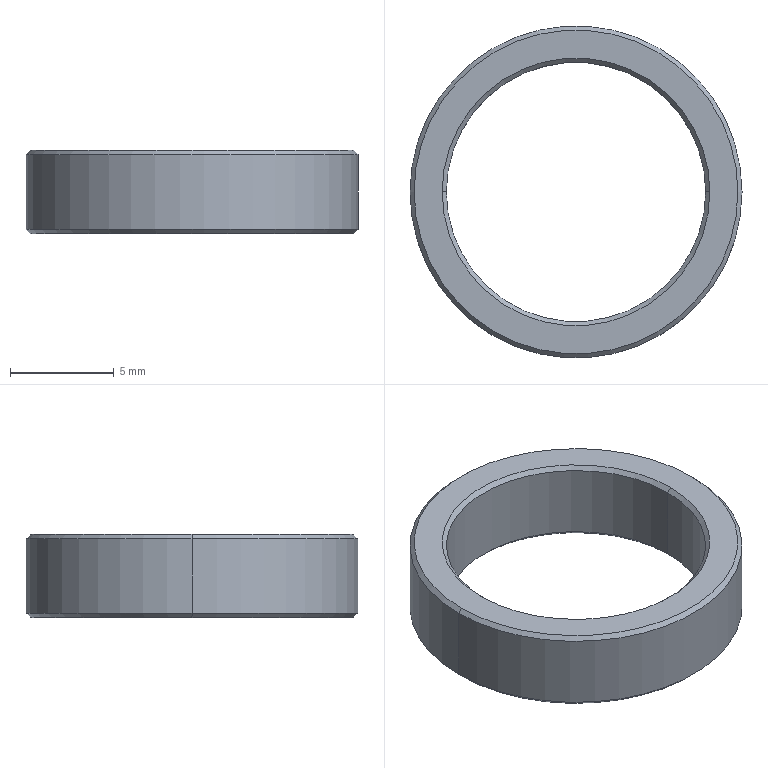Part | SolidWorks | features Chamfer 1, Extrusion 1 | 1 solid | 14 faces | box 16 x 16 x 4 mm | volume 309.792 mm3 | cone 8 | cylinder 4 | plane 2 | commonest cylinder face diameters 12.5 x2 16 x2
STEP:
#1=CARTESIAN_POINT('',(-7.8,0.,-2.));
#2=VERTEX_POINT('',#1);
#3=CARTESIAN_POINT('',(7.8,0.,-2.));
#4=VERTEX_POINT('',#3);
#5=CARTESIAN_POINT('',(0.,0.,-2.));
#6=DIRECTION('',(0.,0.,-1.));
#7=DIRECTION('',(1.,0.,0.));
#8=AXIS2_PLACEMENT_3D('',#5,#6,#7);
#9=CIRCLE('',#8,7.8);
#10=EDGE_CURVE('',#2,#4,#9,.T.);
#11=ORIENTED_EDGE('',*,*,#10,.F.);
#12=CARTESIAN_POINT('',(-8.,0.,-1.8));
#13=VERTEX_POINT('',#12);
#14=CARTESIAN_POINT('',(-8.,0.,-1.8));
#15=DIRECTION('',(-0.7071,0.,0.7071));
#16=VECTOR('',#15,1000.);
#17=LINE('',#14,#16);
#18=EDGE_CURVE('',#2,#13,#17,.T.);
#19=ORIENTED_EDGE('',*,*,#18,.T.);
#20=CARTESIAN_POINT('',(8.,0.,-1.8));
#21=VERTEX_POINT('',#20);
#22=CARTESIAN_POINT('',(0.,0.,-1.8));
#23=DIRECTION('',(0.,0.,1.));
#24=DIRECTION('',(1.,0.,0.));
#25=AXIS2_PLACEMENT_3D('',#22,#23,#24);
#26=CIRCLE('',#25,8.);
#27=EDGE_CURVE('',#21,#13,#26,.T.);
#28=ORIENTED_EDGE('',*,*,#27,.F.);
#29=CARTESIAN_POINT('',(8.,0.,-1.8));
#30=DIRECTION('',(0.7071,0.,0.7071));
#31=VECTOR('',#30,1000.);
#32=LINE('',#29,#31);
#33=EDGE_CURVE('',#4,#21,#32,.T.);
#34=ORIENTED_EDGE('',*,*,#33,.F.);
#35=EDGE_LOOP('',(#11,#19,#28,#34));
#36=FACE_OUTER_BOUND('',#35,.T.);
#37=CARTESIAN_POINT('',(0.,0.,-1.8));
#38=DIRECTION('',(0.,0.,1.));
#39=DIRECTION('',(1.,0.,0.));
#40=AXIS2_PLACEMENT_3D('',#37,#38,#39);
#41=CONICAL_SURFACE('',#40,8.,0.7854);
#42=ADVANCED_FACE('',(#36),#41,.T.);
#43=CARTESIAN_POINT('',(6.25,0.,-1.8));
#44=VERTEX_POINT('',#43);
#45=CARTESIAN_POINT('',(-6.25,0.,-1.8));
#46=VERTEX_POINT('',#45);
#47=CARTESIAN_POINT('',(0.,0.,-1.8));
#48=DIRECTION('',(0.,0.,-1.));
#49=DIRECTION('',(1.,0.,0.));
#50=AXIS2_PLACEMENT_3D('',#47,#48,#49);
#51=CIRCLE('',#50,6.25);
#52=EDGE_CURVE('',#44,#46,#51,.T.);
#53=ORIENTED_EDGE('',*,*,#52,.F.);
#54=CARTESIAN_POINT('',(6.45,0.,-2.));
#55=VERTEX_POINT('',#54);
#56=CARTESIAN_POINT('',(6.45,0.,-2.));
#57=DIRECTION('',(0.7071,0.,-0.7071));
#58=VECTOR('',#57,1000.);
#59=LINE('',#56,#58);
#60=EDGE_CURVE('',#44,#55,#59,.T.);
#61=ORIENTED_EDGE('',*,*,#60,.T.);
#62=CARTESIAN_POINT('',(-6.45,0.,-2.));
#63=VERTEX_POINT('',#62);
#64=CARTESIAN_POINT('',(0.,0.,-2.));
#65=DIRECTION('',(0.,0.,1.));
#66=DIRECTION('',(1.,0.,0.));
#67=AXIS2_PLACEMENT_3D('',#64,#65,#66);
#68=CIRCLE('',#67,6.45);
#69=EDGE_CURVE('',#63,#55,#68,.T.);
#70=ORIENTED_EDGE('',*,*,#69,.F.);
#71=CARTESIAN_POINT('',(-6.45,0.,-2.));
#72=DIRECTION('',(-0.7071,0.,-0.7071));
#73=VECTOR('',#72,1000.);
#74=LINE('',#71,#73);
#75=EDGE_CURVE('',#46,#63,#74,.T.);
#76=ORIENTED_EDGE('',*,*,#75,.F.);
#77=EDGE_LOOP('',(#53,#61,#70,#76));
#78=FACE_OUTER_BOUND('',#77,.T.);
#79=CARTESIAN_POINT('',(0.,0.,-2.));
#80=DIRECTION('',(0.,0.,-1.));
#81=DIRECTION('',(-1.,0.,0.));
#82=AXIS2_PLACEMENT_3D('',#79,#80,#81);
#83=CONICAL_SURFACE('',#82,6.45,0.7854);
#84=ADVANCED_FACE('',(#78),#83,.F.);
#85=CARTESIAN_POINT('',(7.8,0.,2.));
#86=VERTEX_POINT('',#85);
#87=CARTESIAN_POINT('',(-7.8,0.,2.));
#88=VERTEX_POINT('',#87);
#89=CARTESIAN_POINT('',(0.,0.,2.));
#90=DIRECTION('',(0.,0.,1.));
#91=DIRECTION('',(1.,0.,0.));
#92=AXIS2_PLACEMENT_3D('',#89,#90,#91);
#93=CIRCLE('',#92,7.8);
#94=EDGE_CURVE('',#86,#88,#93,.T.);
#95=ORIENTED_EDGE('',*,*,#94,.F.);
#96=CARTESIAN_POINT('',(8.,0.,1.8));
#97=VERTEX_POINT('',#96);
#98=CARTESIAN_POINT('',(7.8,0.,2.));
#99=DIRECTION('',(0.7071,0.,-0.7071));
#100=VECTOR('',#99,1000.);
#101=LINE('',#98,#100);
#102=EDGE_CURVE('',#86,#97,#101,.T.);
#103=ORIENTED_EDGE('',*,*,#102,.T.);
#104=CARTESIAN_POINT('',(-8.,0.,1.8));
#105=VERTEX_POINT('',#104);
#106=CARTESIAN_POINT('',(0.,0.,1.8));
#107=DIRECTION('',(0.,0.,-1.));
#108=DIRECTION('',(1.,0.,0.));
#109=AXIS2_PLACEMENT_3D('',#106,#107,#108);
#110=CIRCLE('',#109,8.);
#111=EDGE_CURVE('',#105,#97,#110,.T.);
#112=ORIENTED_EDGE('',*,*,#111,.F.);
#113=CARTESIAN_POINT('',(-7.8,0.,2.));
#114=DIRECTION('',(-0.7071,0.,-0.7071));
#115=VECTOR('',#114,1000.);
#116=LINE('',#113,#115);
#117=EDGE_CURVE('',#88,#105,#116,.T.);
#118=ORIENTED_EDGE('',*,*,#117,.F.);
#119=EDGE_LOOP('',(#95,#103,#112,#118));
#120=FACE_OUTER_BOUND('',#119,.T.);
#121=CARTESIAN_POINT('',(0.,0.,2.));
#122=DIRECTION('',(0.,0.,-1.));
#123=DIRECTION('',(-1.,0.,0.));
#124=AXIS2_PLACEMENT_3D('',#121,#122,#123);
#125=CONICAL_SURFACE('',#124,7.8,0.7854);
#126=ADVANCED_FACE('',(#120),#125,.T.);
#127=CARTESIAN_POINT('',(-6.25,0.,1.8));
#128=VERTEX_POINT('',#127);
#129=CARTESIAN_POINT('',(6.25,0.,1.8));
#130=VERTEX_POINT('',#129);
#131=CARTESIAN_POINT('',(0.,0.,1.8));
#132=DIRECTION('',(0.,0.,1.));
#133=DIRECTION('',(1.,0.,0.));
#134=AXIS2_PLACEMENT_3D('',#131,#132,#133);
#135=CIRCLE('',#134,6.25);
#136=EDGE_CURVE('',#128,#130,#135,.T.);
#137=ORIENTED_EDGE('',*,*,#136,.F.);
#138=CARTESIAN_POINT('',(-6.45,0.,2.));
#139=VERTEX_POINT('',#138);
#140=CARTESIAN_POINT('',(-6.25,0.,1.8));
#141=DIRECTION('',(-0.7071,0.,0.7071));
#142=VECTOR('',#141,1000.);
#143=LINE('',#140,#142);
#144=EDGE_CURVE('',#128,#139,#143,.T.);
#145=ORIENTED_EDGE('',*,*,#144,.T.);
#146=CARTESIAN_POINT('',(6.45,0.,2.));
#147=VERTEX_POINT('',#146);
#148=CARTESIAN_POINT('',(0.,0.,2.));
#149=DIRECTION('',(0.,0.,-1.));
#150=DIRECTION('',(1.,0.,0.));
#151=AXIS2_PLACEMENT_3D('',#148,#149,#150);
#152=CIRCLE('',#151,6.45);
#153=EDGE_CURVE('',#147,#139,#152,.T.);
#154=ORIENTED_EDGE('',*,*,#153,.F.);
#155=CARTESIAN_POINT('',(6.25,0.,1.8));
#156=DIRECTION('',(0.7071,0.,0.7071));
#157=VECTOR('',#156,1000.);
#158=LINE('',#155,#157);
#159=EDGE_CURVE('',#130,#147,#158,.T.);
#160=ORIENTED_EDGE('',*,*,#159,.F.);
#161=EDGE_LOOP('',(#137,#145,#154,#160));
#162=FACE_OUTER_BOUND('',#161,.T.);
#163=CARTESIAN_POINT('',(0.,0.,1.8));
#164=DIRECTION('',(0.,0.,1.));
#165=DIRECTION('',(1.,0.,0.));
#166=AXIS2_PLACEMENT_3D('',#163,#164,#165);
#167=CONICAL_SURFACE('',#166,6.25,0.7854);
#168=ADVANCED_FACE('',(#162),#167,.F.);
#169=ORIENTED_EDGE('',*,*,#136,.T.);
#170=CARTESIAN_POINT('',(6.25,0.,2.));
#171=DIRECTION('',(0.,0.,-1.));
#172=VECTOR('',#171,1000.);
#173=LINE('',#170,#172);
#174=EDGE_CURVE('',#130,#44,#173,.T.);
#175=ORIENTED_EDGE('',*,*,#174,.T.);
#176=ORIENTED_EDGE('',*,*,#52,.T.);
#177=CARTESIAN_POINT('',(-6.25,0.,2.));
#178=DIRECTION('',(0.,0.,-1.));
#179=VECTOR('',#178,1000.);
#180=LINE('',#177,#179);
#181=EDGE_CURVE('',#128,#46,#180,.T.);
#182=ORIENTED_EDGE('',*,*,#181,.F.);
#183=EDGE_LOOP('',(#169,#175,#176,#182));
#184=FACE_OUTER_BOUND('',#183,.T.);
#185=CARTESIAN_POINT('',(0.,0.,2.));
#186=DIRECTION('',(0.,0.,-1.));
#187=DIRECTION('',(-1.,0.,0.));
#188=AXIS2_PLACEMENT_3D('',#185,#186,#187);
#189=CYLINDRICAL_SURFACE('',#188,6.25);
#190=ADVANCED_FACE('',(#184),#189,.F.);
#191=ORIENTED_EDGE('',*,*,#111,.T.);
#192=CARTESIAN_POINT('',(8.,0.,2.));
#193=DIRECTION('',(0.,0.,-1.));
#194=VECTOR('',#193,1000.);
#195=LINE('',#192,#194);
#196=EDGE_CURVE('',#97,#21,#195,.T.);
#197=ORIENTED_EDGE('',*,*,#196,.T.);
#198=ORIENTED_EDGE('',*,*,#27,.T.);
#199=CARTESIAN_POINT('',(-8.,0.,2.));
#200=DIRECTION('',(0.,0.,-1.));
#201=VECTOR('',#200,1000.);
#202=LINE('',#199,#201);
#203=EDGE_CURVE('',#105,#13,#202,.T.);
#204=ORIENTED_EDGE('',*,*,#203,.F.);
#205=EDGE_LOOP('',(#191,#197,#198,#204));
#206=FACE_OUTER_BOUND('',#205,.T.);
#207=CARTESIAN_POINT('',(0.,0.,2.));
#208=DIRECTION('',(0.,0.,-1.));
#209=DIRECTION('',(-1.,0.,0.));
#210=AXIS2_PLACEMENT_3D('',#207,#208,#209);
#211=CYLINDRICAL_SURFACE('',#210,8.);
#212=ADVANCED_FACE('',(#206),#211,.T.);
#213=ORIENTED_EDGE('',*,*,#153,.T.);
#214=CARTESIAN_POINT('',(0.,0.,2.));
#215=DIRECTION('',(0.,0.,-1.));
#216=DIRECTION('',(1.,0.,0.));
#217=AXIS2_PLACEMENT_3D('',#214,#215,#216);
#218=CIRCLE('',#217,6.45);
#219=EDGE_CURVE('',#139,#147,#218,.T.);
#220=ORIENTED_EDGE('',*,*,#219,.T.);
#221=EDGE_LOOP('',(#213,#220));
#222=FACE_BOUND('',#221,.T.);
#223=CARTESIAN_POINT('',(0.,0.,2.));
#224=DIRECTION('',(0.,0.,1.));
#225=DIRECTION('',(1.,0.,0.));
#226=AXIS2_PLACEMENT_3D('',#223,#224,#225);
#227=CIRCLE('',#226,7.8);
#228=EDGE_CURVE('',#88,#86,#227,.T.);
#229=ORIENTED_EDGE('',*,*,#228,.T.);
#230=ORIENTED_EDGE('',*,*,#94,.T.);
#231=EDGE_LOOP('',(#229,#230));
#232=FACE_OUTER_BOUND('',#231,.T.);
#233=CARTESIAN_POINT('',(0.,0.,2.));
#234=DIRECTION('',(0.,0.,1.));
#235=DIRECTION('',(1.,0.,0.));
#236=AXIS2_PLACEMENT_3D('',#233,#234,#235);
#237=PLANE('',#236);
#238=ADVANCED_FACE('',(#222,#232),#237,.T.);
#239=ORIENTED_EDGE('',*,*,#69,.T.);
#240=CARTESIAN_POINT('',(0.,0.,-2.));
#241=DIRECTION('',(0.,0.,1.));
#242=DIRECTION('',(1.,0.,0.));
#243=AXIS2_PLACEMENT_3D('',#240,#241,#242);
#244=CIRCLE('',#243,6.45);
#245=EDGE_CURVE('',#55,#63,#244,.T.);
#246=ORIENTED_EDGE('',*,*,#245,.T.);
#247=EDGE_LOOP('',(#239,#246));
#248=FACE_BOUND('',#247,.T.);
#249=CARTESIAN_POINT('',(0.,0.,-2.));
#250=DIRECTION('',(0.,0.,-1.));
#251=DIRECTION('',(1.,0.,0.));
#252=AXIS2_PLACEMENT_3D('',#249,#250,#251);
#253=CIRCLE('',#252,7.8);
#254=EDGE_CURVE('',#4,#2,#253,.T.);
#255=ORIENTED_EDGE('',*,*,#254,.T.);
#256=ORIENTED_EDGE('',*,*,#10,.T.);
#257=EDGE_LOOP('',(#255,#256));
#258=FACE_OUTER_BOUND('',#257,.T.);
#259=CARTESIAN_POINT('',(0.,0.,-2.));
#260=DIRECTION('',(0.,0.,1.));
#261=DIRECTION('',(1.,0.,0.));
#262=AXIS2_PLACEMENT_3D('',#259,#260,#261);
#263=PLANE('',#262);
#264=ADVANCED_FACE('',(#248,#258),#263,.F.);
#265=ORIENTED_EDGE('',*,*,#196,.F.);
#266=CARTESIAN_POINT('',(0.,0.,1.8));
#267=DIRECTION('',(0.,0.,-1.));
#268=DIRECTION('',(1.,0.,0.));
#269=AXIS2_PLACEMENT_3D('',#266,#267,#268);
#270=CIRCLE('',#269,8.);
#271=EDGE_CURVE('',#97,#105,#270,.T.);
#272=ORIENTED_EDGE('',*,*,#271,.T.);
#273=ORIENTED_EDGE('',*,*,#203,.T.);
#274=CARTESIAN_POINT('',(0.,0.,-1.8));
#275=DIRECTION('',(0.,0.,1.));
#276=DIRECTION('',(1.,0.,0.));
#277=AXIS2_PLACEMENT_3D('',#274,#275,#276);
#278=CIRCLE('',#277,8.);
#279=EDGE_CURVE('',#13,#21,#278,.T.);
#280=ORIENTED_EDGE('',*,*,#279,.T.);
#281=EDGE_LOOP('',(#265,#272,#273,#280));
#282=FACE_OUTER_BOUND('',#281,.T.);
#283=CARTESIAN_POINT('',(0.,0.,2.));
#284=DIRECTION('',(0.,0.,-1.));
#285=DIRECTION('',(-1.,0.,0.));
#286=AXIS2_PLACEMENT_3D('',#283,#284,#285);
#287=CYLINDRICAL_SURFACE('',#286,8.);
#288=ADVANCED_FACE('',(#282),#287,.T.);
#289=ORIENTED_EDGE('',*,*,#174,.F.);
#290=CARTESIAN_POINT('',(0.,0.,1.8));
#291=DIRECTION('',(0.,0.,1.));
#292=DIRECTION('',(1.,0.,0.));
#293=AXIS2_PLACEMENT_3D('',#290,#291,#292);
#294=CIRCLE('',#293,6.25);
#295=EDGE_CURVE('',#130,#128,#294,.T.);
#296=ORIENTED_EDGE('',*,*,#295,.T.);
#297=ORIENTED_EDGE('',*,*,#181,.T.);
#298=CARTESIAN_POINT('',(0.,0.,-1.8));
#299=DIRECTION('',(0.,0.,-1.));
#300=DIRECTION('',(1.,0.,0.));
#301=AXIS2_PLACEMENT_3D('',#298,#299,#300);
#302=CIRCLE('',#301,6.25);
#303=EDGE_CURVE('',#46,#44,#302,.T.);
#304=ORIENTED_EDGE('',*,*,#303,.T.);
#305=EDGE_LOOP('',(#289,#296,#297,#304));
#306=FACE_OUTER_BOUND('',#305,.T.);
#307=CARTESIAN_POINT('',(0.,0.,2.));
#308=DIRECTION('',(0.,0.,-1.));
#309=DIRECTION('',(-1.,0.,0.));
#310=AXIS2_PLACEMENT_3D('',#307,#308,#309);
#311=CYLINDRICAL_SURFACE('',#310,6.25);
#312=ADVANCED_FACE('',(#306),#311,.F.);
#313=ORIENTED_EDGE('',*,*,#144,.F.);
#314=ORIENTED_EDGE('',*,*,#295,.F.);
#315=ORIENTED_EDGE('',*,*,#159,.T.);
#316=ORIENTED_EDGE('',*,*,#219,.F.);
#317=EDGE_LOOP('',(#313,#314,#315,#316));
#318=FACE_OUTER_BOUND('',#317,.T.);
#319=CARTESIAN_POINT('',(0.,0.,1.8));
#320=DIRECTION('',(0.,0.,1.));
#321=DIRECTION('',(1.,0.,0.));
#322=AXIS2_PLACEMENT_3D('',#319,#320,#321);
#323=CONICAL_SURFACE('',#322,6.25,0.7854);
#324=ADVANCED_FACE('',(#318),#323,.F.);
#325=ORIENTED_EDGE('',*,*,#102,.F.);
#326=ORIENTED_EDGE('',*,*,#228,.F.);
#327=ORIENTED_EDGE('',*,*,#117,.T.);
#328=ORIENTED_EDGE('',*,*,#271,.F.);
#329=EDGE_LOOP('',(#325,#326,#327,#328));
#330=FACE_OUTER_BOUND('',#329,.T.);
#331=CARTESIAN_POINT('',(0.,0.,2.));
#332=DIRECTION('',(0.,0.,-1.));
#333=DIRECTION('',(-1.,0.,0.));
#334=AXIS2_PLACEMENT_3D('',#331,#332,#333);
#335=CONICAL_SURFACE('',#334,7.8,0.7854);
#336=ADVANCED_FACE('',(#330),#335,.T.);
#337=ORIENTED_EDGE('',*,*,#60,.F.);
#338=ORIENTED_EDGE('',*,*,#303,.F.);
#339=ORIENTED_EDGE('',*,*,#75,.T.);
#340=ORIENTED_EDGE('',*,*,#245,.F.);
#341=EDGE_LOOP('',(#337,#338,#339,#340));
#342=FACE_OUTER_BOUND('',#341,.T.);
#343=CARTESIAN_POINT('',(0.,0.,-2.));
#344=DIRECTION('',(0.,0.,-1.));
#345=DIRECTION('',(-1.,0.,0.));
#346=AXIS2_PLACEMENT_3D('',#343,#344,#345);
#347=CONICAL_SURFACE('',#346,6.45,0.7854);
#348=ADVANCED_FACE('',(#342),#347,.F.);
#349=ORIENTED_EDGE('',*,*,#18,.F.);
#350=ORIENTED_EDGE('',*,*,#254,.F.);
#351=ORIENTED_EDGE('',*,*,#33,.T.);
#352=ORIENTED_EDGE('',*,*,#279,.F.);
#353=EDGE_LOOP('',(#349,#350,#351,#352));
#354=FACE_OUTER_BOUND('',#353,.T.);
#355=CARTESIAN_POINT('',(0.,0.,-1.8));
#356=DIRECTION('',(0.,0.,1.));
#357=DIRECTION('',(1.,0.,0.));
#358=AXIS2_PLACEMENT_3D('',#355,#356,#357);
#359=CONICAL_SURFACE('',#358,8.,0.7854);
#360=ADVANCED_FACE('',(#354),#359,.T.);
#361=CLOSED_SHELL('',(#42,#84,#126,#168,#190,#212,#238,#264,#288,#312,#324,#336,#348,#360));
#362=MANIFOLD_SOLID_BREP('',#361);
#363=CARTESIAN_POINT('',(0.,0.,0.));
#364=DIRECTION('',(0.,0.,1.));
#365=DIRECTION('',(1.,0.,0.));
#366=AXIS2_PLACEMENT_3D('',#363,#364,#365);
#367=(LENGTH_UNIT()NAMED_UNIT(*)SI_UNIT(.MILLI.,.METRE.));
#368=UNCERTAINTY_MEASURE_WITH_UNIT(LENGTH_MEASURE(0.00001),#367,'','');
#369=(NAMED_UNIT(*)PLANE_ANGLE_UNIT()SI_UNIT($,.RADIAN.));
#370=(NAMED_UNIT(*)SI_UNIT($,.STERADIAN.)SOLID_ANGLE_UNIT());
#371=(GEOMETRIC_REPRESENTATION_CONTEXT(3)GLOBAL_UNCERTAINTY_ASSIGNED_CONTEXT((#368))GLOBAL_UNIT_ASSIGNED_CONTEXT((#367,#369,#370))REPRESENTATION_CONTEXT('',''));
#372=ADVANCED_BREP_SHAPE_REPRESENTATION('',(#362,#366),#371);